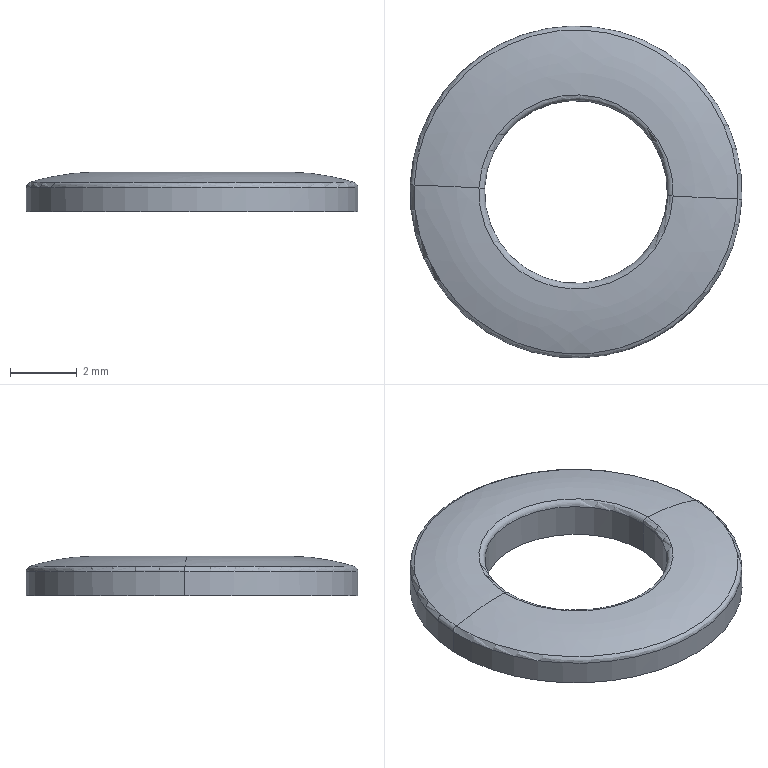Part | SolidWorks | features BaseBody 1 | 1 solid | 11 faces | box 9.985 x 9.985 x 1.184 mm | volume 57.779 mm3 | cylinder 4 | torus 4 | spline 2 | plane 1 | commonest cylinder face diameters 5.5 x2 9.985 x2
STEP:
#1=CARTESIAN_POINT('',(-14.747,-20.881,-9.184));
#2=VERTEX_POINT('',#1);
#3=CARTESIAN_POINT('',(-9.253,-21.119,-9.184));
#4=VERTEX_POINT('',#3);
#5=CARTESIAN_POINT('',(-12.,-21.,-9.184));
#6=DIRECTION('',(0.,0.,-1.));
#7=DIRECTION('',(-0.9991,0.0431,0.));
#8=AXIS2_PLACEMENT_3D('',#5,#6,#7);
#9=CIRCLE('',#8,2.75);
#10=EDGE_CURVE('',#2,#4,#9,.T.);
#11=ORIENTED_EDGE('',*,*,#10,.T.);
#12=CARTESIAN_POINT('',(-9.253,-21.119,-8.169));
#13=VERTEX_POINT('',#12);
#14=CARTESIAN_POINT('',(-9.253,-21.119,-8.169));
#15=DIRECTION('',(0.,0.,-1.));
#16=VECTOR('',#15,1000.);
#17=LINE('',#14,#16);
#18=EDGE_CURVE('',#13,#4,#17,.T.);
#19=ORIENTED_EDGE('',*,*,#18,.F.);
#20=CARTESIAN_POINT('',(-9.252,-21.104,-8.169));
#21=VERTEX_POINT('',#20);
#22=CARTESIAN_POINT('',(-12.,-21.,-8.169));
#23=DIRECTION('',(0.,0.,1.));
#24=DIRECTION('',(0.9991,-0.0431,0.));
#25=AXIS2_PLACEMENT_3D('',#22,#23,#24);
#26=CIRCLE('',#25,2.75);
#27=EDGE_CURVE('',#13,#21,#26,.T.);
#28=ORIENTED_EDGE('',*,*,#27,.T.);
#29=CARTESIAN_POINT('',(-14.747,-20.881,-8.169));
#30=VERTEX_POINT('',#29);
#31=CARTESIAN_POINT('',(-12.,-21.,-8.169));
#32=DIRECTION('',(0.,0.,1.));
#33=DIRECTION('',(0.9993,-0.0378,0.));
#34=AXIS2_PLACEMENT_3D('',#31,#32,#33);
#35=CIRCLE('',#34,2.75);
#36=EDGE_CURVE('',#21,#30,#35,.T.);
#37=ORIENTED_EDGE('',*,*,#36,.T.);
#38=CARTESIAN_POINT('',(-14.747,-20.881,-8.169));
#39=DIRECTION('',(0.,0.,-1.));
#40=VECTOR('',#39,1000.);
#41=LINE('',#38,#40);
#42=EDGE_CURVE('',#30,#2,#41,.T.);
#43=ORIENTED_EDGE('',*,*,#42,.T.);
#44=EDGE_LOOP('',(#11,#19,#28,#37,#43));
#45=FACE_OUTER_BOUND('',#44,.T.);
#46=CARTESIAN_POINT('',(-12.,-21.,-9.184));
#47=DIRECTION('',(0.,0.,1.));
#48=DIRECTION('',(0.9991,-0.0431,0.));
#49=AXIS2_PLACEMENT_3D('',#46,#47,#48);
#50=CYLINDRICAL_SURFACE('',#49,2.75);
#51=ADVANCED_FACE('',(#45),#50,.F.);
#52=ORIENTED_EDGE('',*,*,#42,.F.);
#53=CARTESIAN_POINT('',(-14.748,-20.896,-8.169));
#54=VERTEX_POINT('',#53);
#55=CARTESIAN_POINT('',(-12.,-21.,-8.169));
#56=DIRECTION('',(0.,0.,1.));
#57=DIRECTION('',(-0.9991,0.0431,0.));
#58=AXIS2_PLACEMENT_3D('',#55,#56,#57);
#59=CIRCLE('',#58,2.75);
#60=EDGE_CURVE('',#30,#54,#59,.T.);
#61=ORIENTED_EDGE('',*,*,#60,.T.);
#62=CARTESIAN_POINT('',(-12.,-21.,-8.169));
#63=DIRECTION('',(0.,0.,1.));
#64=DIRECTION('',(-0.9993,0.0378,0.));
#65=AXIS2_PLACEMENT_3D('',#62,#63,#64);
#66=CIRCLE('',#65,2.75);
#67=EDGE_CURVE('',#54,#13,#66,.T.);
#68=ORIENTED_EDGE('',*,*,#67,.T.);
#69=ORIENTED_EDGE('',*,*,#18,.T.);
#70=CARTESIAN_POINT('',(-12.,-21.,-9.184));
#71=DIRECTION('',(0.,0.,-1.));
#72=DIRECTION('',(0.9991,-0.0431,0.));
#73=AXIS2_PLACEMENT_3D('',#70,#71,#72);
#74=CIRCLE('',#73,2.75);
#75=EDGE_CURVE('',#4,#2,#74,.T.);
#76=ORIENTED_EDGE('',*,*,#75,.T.);
#77=EDGE_LOOP('',(#52,#61,#68,#69,#76));
#78=FACE_OUTER_BOUND('',#77,.T.);
#79=CARTESIAN_POINT('',(-12.,-21.,-9.184));
#80=DIRECTION('',(0.,0.,1.));
#81=DIRECTION('',(0.9991,-0.0431,0.));
#82=AXIS2_PLACEMENT_3D('',#79,#80,#81);
#83=CYLINDRICAL_SURFACE('',#82,2.75);
#84=ADVANCED_FACE('',(#78),#83,.F.);
#85=ORIENTED_EDGE('',*,*,#10,.F.);
#86=ORIENTED_EDGE('',*,*,#75,.F.);
#87=EDGE_LOOP('',(#85,#86));
#88=FACE_BOUND('',#87,.T.);
#89=CARTESIAN_POINT('',(-16.988,-20.785,-9.184));
#90=VERTEX_POINT('',#89);
#91=CARTESIAN_POINT('',(-7.012,-21.215,-9.184));
#92=VERTEX_POINT('',#91);
#93=CARTESIAN_POINT('',(-12.,-21.,-9.184));
#94=DIRECTION('',(0.,0.,1.));
#95=DIRECTION('',(-0.9991,0.0431,0.));
#96=AXIS2_PLACEMENT_3D('',#93,#94,#95);
#97=CIRCLE('',#96,4.992);
#98=EDGE_CURVE('',#90,#92,#97,.T.);
#99=ORIENTED_EDGE('',*,*,#98,.F.);
#100=CARTESIAN_POINT('',(-12.,-21.,-9.184));
#101=DIRECTION('',(0.,0.,1.));
#102=DIRECTION('',(0.9991,-0.0431,0.));
#103=AXIS2_PLACEMENT_3D('',#100,#101,#102);
#104=CIRCLE('',#103,4.992);
#105=EDGE_CURVE('',#92,#90,#104,.T.);
#106=ORIENTED_EDGE('',*,*,#105,.F.);
#107=EDGE_LOOP('',(#99,#106));
#108=FACE_OUTER_BOUND('',#107,.T.);
#109=CARTESIAN_POINT('',(-12.,-21.,-9.184));
#110=DIRECTION('',(0.,0.,1.));
#111=DIRECTION('',(1.,0.,0.));
#112=AXIS2_PLACEMENT_3D('',#109,#110,#111);
#113=PLANE('',#112);
#114=ADVANCED_FACE('',(#88,#108),#113,.F.);
#115=CARTESIAN_POINT('',(-16.988,-20.785,-8.462));
#116=VERTEX_POINT('',#115);
#117=CARTESIAN_POINT('',(-16.988,-20.785,-8.462));
#118=DIRECTION('',(0.,0.,-1.));
#119=VECTOR('',#118,1000.);
#120=LINE('',#117,#119);
#121=EDGE_CURVE('',#116,#90,#120,.T.);
#122=ORIENTED_EDGE('',*,*,#121,.F.);
#123=CARTESIAN_POINT('',(-16.987,-20.763,-8.462));
#124=VERTEX_POINT('',#123);
#125=CARTESIAN_POINT('',(-12.,-21.,-8.462));
#126=DIRECTION('',(0.,0.,-1.));
#127=DIRECTION('',(-0.9991,0.0431,0.));
#128=AXIS2_PLACEMENT_3D('',#125,#126,#127);
#129=CIRCLE('',#128,4.992);
#130=EDGE_CURVE('',#116,#124,#129,.T.);
#131=ORIENTED_EDGE('',*,*,#130,.T.);
#132=CARTESIAN_POINT('',(-7.012,-21.215,-8.462));
#133=VERTEX_POINT('',#132);
#134=CARTESIAN_POINT('',(-12.,-21.,-8.462));
#135=DIRECTION('',(0.,0.,-1.));
#136=DIRECTION('',(-0.9989,0.04746,0.));
#137=AXIS2_PLACEMENT_3D('',#134,#135,#136);
#138=CIRCLE('',#137,4.992);
#139=EDGE_CURVE('',#124,#133,#138,.T.);
#140=ORIENTED_EDGE('',*,*,#139,.T.);
#141=CARTESIAN_POINT('',(-7.012,-21.215,-8.462));
#142=DIRECTION('',(0.,0.,-1.));
#143=VECTOR('',#142,1000.);
#144=LINE('',#141,#143);
#145=EDGE_CURVE('',#133,#92,#144,.T.);
#146=ORIENTED_EDGE('',*,*,#145,.T.);
#147=ORIENTED_EDGE('',*,*,#105,.T.);
#148=EDGE_LOOP('',(#122,#131,#140,#146,#147));
#149=FACE_OUTER_BOUND('',#148,.T.);
#150=CARTESIAN_POINT('',(-12.,-21.,-9.184));
#151=DIRECTION('',(0.,0.,1.));
#152=DIRECTION('',(0.9991,-0.0431,0.));
#153=AXIS2_PLACEMENT_3D('',#150,#151,#152);
#154=CYLINDRICAL_SURFACE('',#153,4.992);
#155=ADVANCED_FACE('',(#149),#154,.T.);
#156=ORIENTED_EDGE('',*,*,#98,.T.);
#157=ORIENTED_EDGE('',*,*,#145,.F.);
#158=CARTESIAN_POINT('',(-7.013,-21.237,-8.462));
#159=VERTEX_POINT('',#158);
#160=CARTESIAN_POINT('',(-12.,-21.,-8.462));
#161=DIRECTION('',(0.,0.,-1.));
#162=DIRECTION('',(0.9991,-0.0431,0.));
#163=AXIS2_PLACEMENT_3D('',#160,#161,#162);
#164=CIRCLE('',#163,4.992);
#165=EDGE_CURVE('',#133,#159,#164,.T.);
#166=ORIENTED_EDGE('',*,*,#165,.T.);
#167=CARTESIAN_POINT('',(-12.,-21.,-8.462));
#168=DIRECTION('',(0.,0.,-1.));
#169=DIRECTION('',(0.9989,-0.04746,0.));
#170=AXIS2_PLACEMENT_3D('',#167,#168,#169);
#171=CIRCLE('',#170,4.992);
#172=EDGE_CURVE('',#159,#116,#171,.T.);
#173=ORIENTED_EDGE('',*,*,#172,.T.);
#174=ORIENTED_EDGE('',*,*,#121,.T.);
#175=EDGE_LOOP('',(#156,#157,#166,#173,#174));
#176=FACE_OUTER_BOUND('',#175,.T.);
#177=CARTESIAN_POINT('',(-12.,-21.,-9.184));
#178=DIRECTION('',(0.,0.,1.));
#179=DIRECTION('',(0.9991,-0.0431,0.));
#180=AXIS2_PLACEMENT_3D('',#177,#178,#179);
#181=CYLINDRICAL_SURFACE('',#180,4.992);
#182=ADVANCED_FACE('',(#176),#181,.T.);
#183=CARTESIAN_POINT('',(-7.133,-21.231,-8.3));
#184=VERTEX_POINT('',#183);
#185=CARTESIAN_POINT('',(-16.868,-20.79,-8.3));
#186=VERTEX_POINT('',#185);
#187=CARTESIAN_POINT('',(-12.,-21.,-8.3));
#188=DIRECTION('',(0.,0.,-1.));
#189=DIRECTION('',(0.9989,-0.04746,0.));
#190=AXIS2_PLACEMENT_3D('',#187,#188,#189);
#191=CIRCLE('',#190,4.873);
#192=EDGE_CURVE('',#184,#186,#191,.T.);
#193=ORIENTED_EDGE('',*,*,#192,.T.);
#194=CARTESIAN_POINT('',(-16.867,-20.769,-8.3));
#195=VERTEX_POINT('',#194);
#196=CARTESIAN_POINT('',(-12.,-21.,-8.3));
#197=DIRECTION('',(0.,0.,-1.));
#198=DIRECTION('',(-0.9991,0.0431,0.));
#199=AXIS2_PLACEMENT_3D('',#196,#197,#198);
#200=CIRCLE('',#199,4.873);
#201=EDGE_CURVE('',#186,#195,#200,.T.);
#202=ORIENTED_EDGE('',*,*,#201,.T.);
#203=CARTESIAN_POINT('',(-16.818,-20.771,-8.462));
#204=DIRECTION('',(0.04746,0.9989,0.));
#205=DIRECTION('',(-0.9989,0.04746,0.));
#206=AXIS2_PLACEMENT_3D('',#203,#204,#205);
#207=CIRCLE('',#206,0.1692);
#208=EDGE_CURVE('',#124,#195,#207,.T.);
#209=ORIENTED_EDGE('',*,*,#208,.F.);
#210=ORIENTED_EDGE('',*,*,#130,.F.);
#211=ORIENTED_EDGE('',*,*,#172,.F.);
#212=CARTESIAN_POINT('',(-7.182,-21.229,-8.462));
#213=DIRECTION('',(-0.04746,-0.9989,0.));
#214=DIRECTION('',(0.9989,-0.04746,0.));
#215=AXIS2_PLACEMENT_3D('',#212,#213,#214);
#216=CIRCLE('',#215,0.1692);
#217=EDGE_CURVE('',#159,#184,#216,.T.);
#218=ORIENTED_EDGE('',*,*,#217,.T.);
#219=EDGE_LOOP('',(#193,#202,#209,#210,#211,#218));
#220=FACE_OUTER_BOUND('',#219,.T.);
#221=CARTESIAN_POINT('',(-12.,-21.,-8.462));
#222=DIRECTION('',(0.,0.,-1.));
#223=DIRECTION('',(-0.9989,0.04746,0.));
#224=AXIS2_PLACEMENT_3D('',#221,#222,#223);
#225=TOROIDAL_SURFACE('',#224,4.823,0.1692);
#226=ADVANCED_FACE('',(#220),#225,.T.);
#227=ORIENTED_EDGE('',*,*,#217,.F.);
#228=ORIENTED_EDGE('',*,*,#165,.F.);
#229=ORIENTED_EDGE('',*,*,#139,.F.);
#230=ORIENTED_EDGE('',*,*,#208,.T.);
#231=CARTESIAN_POINT('',(-7.132,-21.21,-8.3));
#232=VERTEX_POINT('',#231);
#233=CARTESIAN_POINT('',(-12.,-21.,-8.3));
#234=DIRECTION('',(0.,0.,-1.));
#235=DIRECTION('',(-0.9989,0.04746,0.));
#236=AXIS2_PLACEMENT_3D('',#233,#234,#235);
#237=CIRCLE('',#236,4.873);
#238=EDGE_CURVE('',#195,#232,#237,.T.);
#239=ORIENTED_EDGE('',*,*,#238,.T.);
#240=CARTESIAN_POINT('',(-12.,-21.,-8.3));
#241=DIRECTION('',(0.,0.,-1.));
#242=DIRECTION('',(0.9991,-0.0431,0.));
#243=AXIS2_PLACEMENT_3D('',#240,#241,#242);
#244=CIRCLE('',#243,4.873);
#245=EDGE_CURVE('',#232,#184,#244,.T.);
#246=ORIENTED_EDGE('',*,*,#245,.T.);
#247=EDGE_LOOP('',(#227,#228,#229,#230,#239,#246));
#248=FACE_OUTER_BOUND('',#247,.T.);
#249=CARTESIAN_POINT('',(-12.,-21.,-8.462));
#250=DIRECTION('',(0.,0.,-1.));
#251=DIRECTION('',(0.9989,-0.04746,0.));
#252=AXIS2_PLACEMENT_3D('',#249,#250,#251);
#253=TOROIDAL_SURFACE('',#252,4.823,0.1692);
#254=ADVANCED_FACE('',(#248),#253,.T.);
#255=CARTESIAN_POINT('',(-14.918,-20.89,-8.));
#256=VERTEX_POINT('',#255);
#257=CARTESIAN_POINT('',(-9.082,-21.126,-8.));
#258=VERTEX_POINT('',#257);
#259=CARTESIAN_POINT('',(-12.,-21.,-8.));
#260=DIRECTION('',(0.,0.,1.));
#261=DIRECTION('',(-0.9993,0.03779,0.));
#262=AXIS2_PLACEMENT_3D('',#259,#260,#261);
#263=CIRCLE('',#262,2.92);
#264=EDGE_CURVE('',#256,#258,#263,.T.);
#265=ORIENTED_EDGE('',*,*,#264,.F.);
#266=CARTESIAN_POINT('',(-14.918,-20.874,-8.));
#267=VERTEX_POINT('',#266);
#268=CARTESIAN_POINT('',(-12.,-21.,-8.));
#269=DIRECTION('',(0.,0.,1.));
#270=DIRECTION('',(-0.9991,0.0431,0.));
#271=AXIS2_PLACEMENT_3D('',#268,#269,#270);
#272=CIRCLE('',#271,2.92);
#273=EDGE_CURVE('',#267,#256,#272,.T.);
#274=ORIENTED_EDGE('',*,*,#273,.F.);
#275=CARTESIAN_POINT('',(-14.874,-20.876,-14.78));
#276=DIRECTION('',(0.0431,0.9991,0.));
#277=DIRECTION('',(-0.2941,0.01269,0.9557));
#278=AXIS2_PLACEMENT_3D('',#275,#276,#277);
#279=CIRCLE('',#278,6.78);
#280=EDGE_CURVE('',#186,#267,#279,.T.);
#281=ORIENTED_EDGE('',*,*,#280,.F.);
#282=ORIENTED_EDGE('',*,*,#192,.F.);
#283=ORIENTED_EDGE('',*,*,#245,.F.);
#284=CARTESIAN_POINT('',(-9.126,-21.124,-14.78));
#285=DIRECTION('',(-0.0431,-0.9991,0.));
#286=DIRECTION('',(0.2941,-0.01269,0.9557));
#287=AXIS2_PLACEMENT_3D('',#284,#285,#286);
#288=CIRCLE('',#287,6.78);
#289=EDGE_CURVE('',#232,#258,#288,.T.);
#290=ORIENTED_EDGE('',*,*,#289,.T.);
#291=EDGE_LOOP('',(#265,#274,#281,#282,#283,#290));
#292=FACE_OUTER_BOUND('',#291,.T.);
#293=CARTESIAN_POINT('',(-9.2,-20.945,-8.));
#294=CARTESIAN_POINT('',(-8.456,-20.93,-7.992));
#295=CARTESIAN_POINT('',(-7.721,-20.916,-8.105));
#296=CARTESIAN_POINT('',(-7.014,-20.902,-8.337));
#297=CARTESIAN_POINT('',(-9.166,-22.668,-8.));
#298=CARTESIAN_POINT('',(-8.413,-23.111,-7.992));
#299=CARTESIAN_POINT('',(-7.669,-23.549,-8.105));
#300=CARTESIAN_POINT('',(-6.953,-23.97,-8.337));
#301=CARTESIAN_POINT('',(-10.399,-23.872,-8.));
#302=CARTESIAN_POINT('',(-9.974,-24.635,-7.992));
#303=CARTESIAN_POINT('',(-9.553,-25.39,-8.105));
#304=CARTESIAN_POINT('',(-9.149,-26.115,-8.337));
#305=CARTESIAN_POINT('',(-12.121,-23.798,-8.));
#306=CARTESIAN_POINT('',(-12.153,-24.541,-7.992));
#307=CARTESIAN_POINT('',(-12.184,-25.276,-8.105));
#308=CARTESIAN_POINT('',(-12.215,-25.983,-8.337));
#309=CARTESIAN_POINT('',(-13.842,-23.723,-8.));
#310=CARTESIAN_POINT('',(-14.332,-24.447,-7.992));
#311=CARTESIAN_POINT('',(-14.816,-25.163,-8.105));
#312=CARTESIAN_POINT('',(-15.281,-25.85,-8.337));
#313=CARTESIAN_POINT('',(-14.967,-22.418,-8.));
#314=CARTESIAN_POINT('',(-15.755,-22.794,-7.992));
#315=CARTESIAN_POINT('',(-16.535,-23.167,-8.105));
#316=CARTESIAN_POINT('',(-17.284,-23.525,-8.337));
#317=CARTESIAN_POINT('',(-14.785,-20.704,-8.));
#318=CARTESIAN_POINT('',(-15.525,-20.625,-7.992));
#319=CARTESIAN_POINT('',(-16.256,-20.547,-8.105));
#320=CARTESIAN_POINT('',(-16.959,-20.473,-8.337));
#321=(BOUNDED_SURFACE()B_SPLINE_SURFACE(3,3,((#293,#294,#295,#296),(#297,#298,#299,#300),(#301,#302,#303,#304),(#305,#306,#307,#308),(#309,#310,#311,#312),(#313,#314,#315,#316),(#317,#318,#319,#320)),.UNSPECIFIED.,.F.,.F.,.T.)B_SPLINE_SURFACE_WITH_KNOTS((4,3,4),(4,4),(0.,1.,2.),(0.,1.),.UNSPECIFIED.)GEOMETRIC_REPRESENTATION_ITEM()RATIONAL_B_SPLINE_SURFACE(((1.195,1.185,1.185,1.195),(0.9439,0.9355,0.9355,0.9439),(0.9439,0.9355,0.9355,0.9439),(1.195,1.185,1.185,1.195),(0.9439,0.9355,0.9355,0.9439),(0.9439,0.9355,0.9355,0.9439),(1.195,1.185,1.185,1.195)))REPRESENTATION_ITEM('')SURFACE());
#322=ADVANCED_FACE('',(#292),#321,.T.);
#323=ORIENTED_EDGE('',*,*,#289,.F.);
#324=ORIENTED_EDGE('',*,*,#238,.F.);
#325=ORIENTED_EDGE('',*,*,#201,.F.);
#326=ORIENTED_EDGE('',*,*,#280,.T.);
#327=CARTESIAN_POINT('',(-9.082,-21.11,-8.));
#328=VERTEX_POINT('',#327);
#329=CARTESIAN_POINT('',(-12.,-21.,-8.));
#330=DIRECTION('',(0.,0.,1.));
#331=DIRECTION('',(0.9993,-0.03779,0.));
#332=AXIS2_PLACEMENT_3D('',#329,#330,#331);
#333=CIRCLE('',#332,2.92);
#334=EDGE_CURVE('',#328,#267,#333,.T.);
#335=ORIENTED_EDGE('',*,*,#334,.F.);
#336=CARTESIAN_POINT('',(-12.,-21.,-8.));
#337=DIRECTION('',(0.,0.,1.));
#338=DIRECTION('',(0.9991,-0.0431,0.));
#339=AXIS2_PLACEMENT_3D('',#336,#337,#338);
#340=CIRCLE('',#339,2.92);
#341=EDGE_CURVE('',#258,#328,#340,.T.);
#342=ORIENTED_EDGE('',*,*,#341,.F.);
#343=EDGE_LOOP('',(#323,#324,#325,#326,#335,#342));
#344=FACE_OUTER_BOUND('',#343,.T.);
#345=CARTESIAN_POINT('',(-14.8,-21.055,-8.));
#346=CARTESIAN_POINT('',(-15.544,-21.07,-7.992));
#347=CARTESIAN_POINT('',(-16.279,-21.084,-8.105));
#348=CARTESIAN_POINT('',(-16.986,-21.098,-8.337));
#349=CARTESIAN_POINT('',(-14.834,-19.332,-8.));
#350=CARTESIAN_POINT('',(-15.587,-18.889,-7.992));
#351=CARTESIAN_POINT('',(-16.331,-18.451,-8.105));
#352=CARTESIAN_POINT('',(-17.047,-18.03,-8.337));
#353=CARTESIAN_POINT('',(-13.601,-18.128,-8.));
#354=CARTESIAN_POINT('',(-14.026,-17.365,-7.992));
#355=CARTESIAN_POINT('',(-14.447,-16.61,-8.105));
#356=CARTESIAN_POINT('',(-14.851,-15.885,-8.337));
#357=CARTESIAN_POINT('',(-11.879,-18.202,-8.));
#358=CARTESIAN_POINT('',(-11.847,-17.459,-7.992));
#359=CARTESIAN_POINT('',(-11.816,-16.724,-8.105));
#360=CARTESIAN_POINT('',(-11.785,-16.017,-8.337));
#361=CARTESIAN_POINT('',(-10.158,-18.277,-8.));
#362=CARTESIAN_POINT('',(-9.668,-17.553,-7.992));
#363=CARTESIAN_POINT('',(-9.184,-16.837,-8.105));
#364=CARTESIAN_POINT('',(-8.719,-16.15,-8.337));
#365=CARTESIAN_POINT('',(-9.033,-19.582,-8.));
#366=CARTESIAN_POINT('',(-8.245,-19.206,-7.992));
#367=CARTESIAN_POINT('',(-7.465,-18.833,-8.105));
#368=CARTESIAN_POINT('',(-6.716,-18.475,-8.337));
#369=CARTESIAN_POINT('',(-9.215,-21.296,-8.));
#370=CARTESIAN_POINT('',(-8.475,-21.375,-7.992));
#371=CARTESIAN_POINT('',(-7.744,-21.453,-8.105));
#372=CARTESIAN_POINT('',(-7.041,-21.527,-8.337));
#373=(BOUNDED_SURFACE()B_SPLINE_SURFACE(3,3,((#345,#346,#347,#348),(#349,#350,#351,#352),(#353,#354,#355,#356),(#357,#358,#359,#360),(#361,#362,#363,#364),(#365,#366,#367,#368),(#369,#370,#371,#372)),.UNSPECIFIED.,.F.,.F.,.F.)B_SPLINE_SURFACE_WITH_KNOTS((4,3,4),(4,4),(0.,1.,2.),(0.,1.),.UNSPECIFIED.)GEOMETRIC_REPRESENTATION_ITEM()RATIONAL_B_SPLINE_SURFACE(((1.195,1.185,1.185,1.195),(0.9439,0.9355,0.9355,0.9439),(0.9439,0.9355,0.9355,0.9439),(1.195,1.185,1.185,1.195),(0.9439,0.9355,0.9355,0.9439),(0.9439,0.9355,0.9355,0.9439),(1.195,1.185,1.185,1.195)))REPRESENTATION_ITEM('')SURFACE());
#374=ADVANCED_FACE('',(#344),#373,.T.);
#375=ORIENTED_EDGE('',*,*,#27,.F.);
#376=ORIENTED_EDGE('',*,*,#67,.F.);
#377=CARTESIAN_POINT('',(-14.917,-20.89,-8.169));
#378=DIRECTION('',(0.0378,0.9993,0.));
#379=DIRECTION('',(-0.006377,0.0002412,1.));
#380=AXIS2_PLACEMENT_3D('',#377,#378,#379);
#381=CIRCLE('',#380,0.1692);
#382=EDGE_CURVE('',#256,#54,#381,.T.);
#383=ORIENTED_EDGE('',*,*,#382,.F.);
#384=ORIENTED_EDGE('',*,*,#264,.T.);
#385=ORIENTED_EDGE('',*,*,#341,.T.);
#386=CARTESIAN_POINT('',(-9.083,-21.11,-8.169));
#387=DIRECTION('',(-0.0378,-0.9993,0.));
#388=DIRECTION('',(0.006377,-0.0002412,1.));
#389=AXIS2_PLACEMENT_3D('',#386,#387,#388);
#390=CIRCLE('',#389,0.1692);
#391=EDGE_CURVE('',#328,#21,#390,.T.);
#392=ORIENTED_EDGE('',*,*,#391,.T.);
#393=EDGE_LOOP('',(#375,#376,#383,#384,#385,#392));
#394=FACE_OUTER_BOUND('',#393,.T.);
#395=CARTESIAN_POINT('',(-12.,-21.,-8.169));
#396=DIRECTION('',(0.,0.,1.));
#397=DIRECTION('',(-0.9993,0.0378,0.));
#398=AXIS2_PLACEMENT_3D('',#395,#396,#397);
#399=TOROIDAL_SURFACE('',#398,2.919,0.1692);
#400=ADVANCED_FACE('',(#394),#399,.T.);
#401=ORIENTED_EDGE('',*,*,#391,.F.);
#402=ORIENTED_EDGE('',*,*,#334,.T.);
#403=ORIENTED_EDGE('',*,*,#273,.T.);
#404=ORIENTED_EDGE('',*,*,#382,.T.);
#405=ORIENTED_EDGE('',*,*,#60,.F.);
#406=ORIENTED_EDGE('',*,*,#36,.F.);
#407=EDGE_LOOP('',(#401,#402,#403,#404,#405,#406));
#408=FACE_OUTER_BOUND('',#407,.T.);
#409=CARTESIAN_POINT('',(-12.,-21.,-8.169));
#410=DIRECTION('',(0.,0.,1.));
#411=DIRECTION('',(0.9993,-0.0378,0.));
#412=AXIS2_PLACEMENT_3D('',#409,#410,#411);
#413=TOROIDAL_SURFACE('',#412,2.919,0.1692);
#414=ADVANCED_FACE('',(#408),#413,.T.);
#415=CLOSED_SHELL('',(#51,#84,#114,#155,#182,#226,#254,#322,#374,#400,#414));
#416=MANIFOLD_SOLID_BREP('',#415);
#417=CARTESIAN_POINT('',(0.,0.,0.));
#418=DIRECTION('',(0.,0.,1.));
#419=DIRECTION('',(1.,0.,0.));
#420=AXIS2_PLACEMENT_3D('',#417,#418,#419);
#421=(LENGTH_UNIT()NAMED_UNIT(*)SI_UNIT(.MILLI.,.METRE.));
#422=UNCERTAINTY_MEASURE_WITH_UNIT(LENGTH_MEASURE(0.00001),#421,'','');
#423=(NAMED_UNIT(*)PLANE_ANGLE_UNIT()SI_UNIT($,.RADIAN.));
#424=(NAMED_UNIT(*)SI_UNIT($,.STERADIAN.)SOLID_ANGLE_UNIT());
#425=(GEOMETRIC_REPRESENTATION_CONTEXT(3)GLOBAL_UNCERTAINTY_ASSIGNED_CONTEXT((#422))GLOBAL_UNIT_ASSIGNED_CONTEXT((#421,#423,#424))REPRESENTATION_CONTEXT('',''));
#426=ADVANCED_BREP_SHAPE_REPRESENTATION('',(#416,#420),#425);